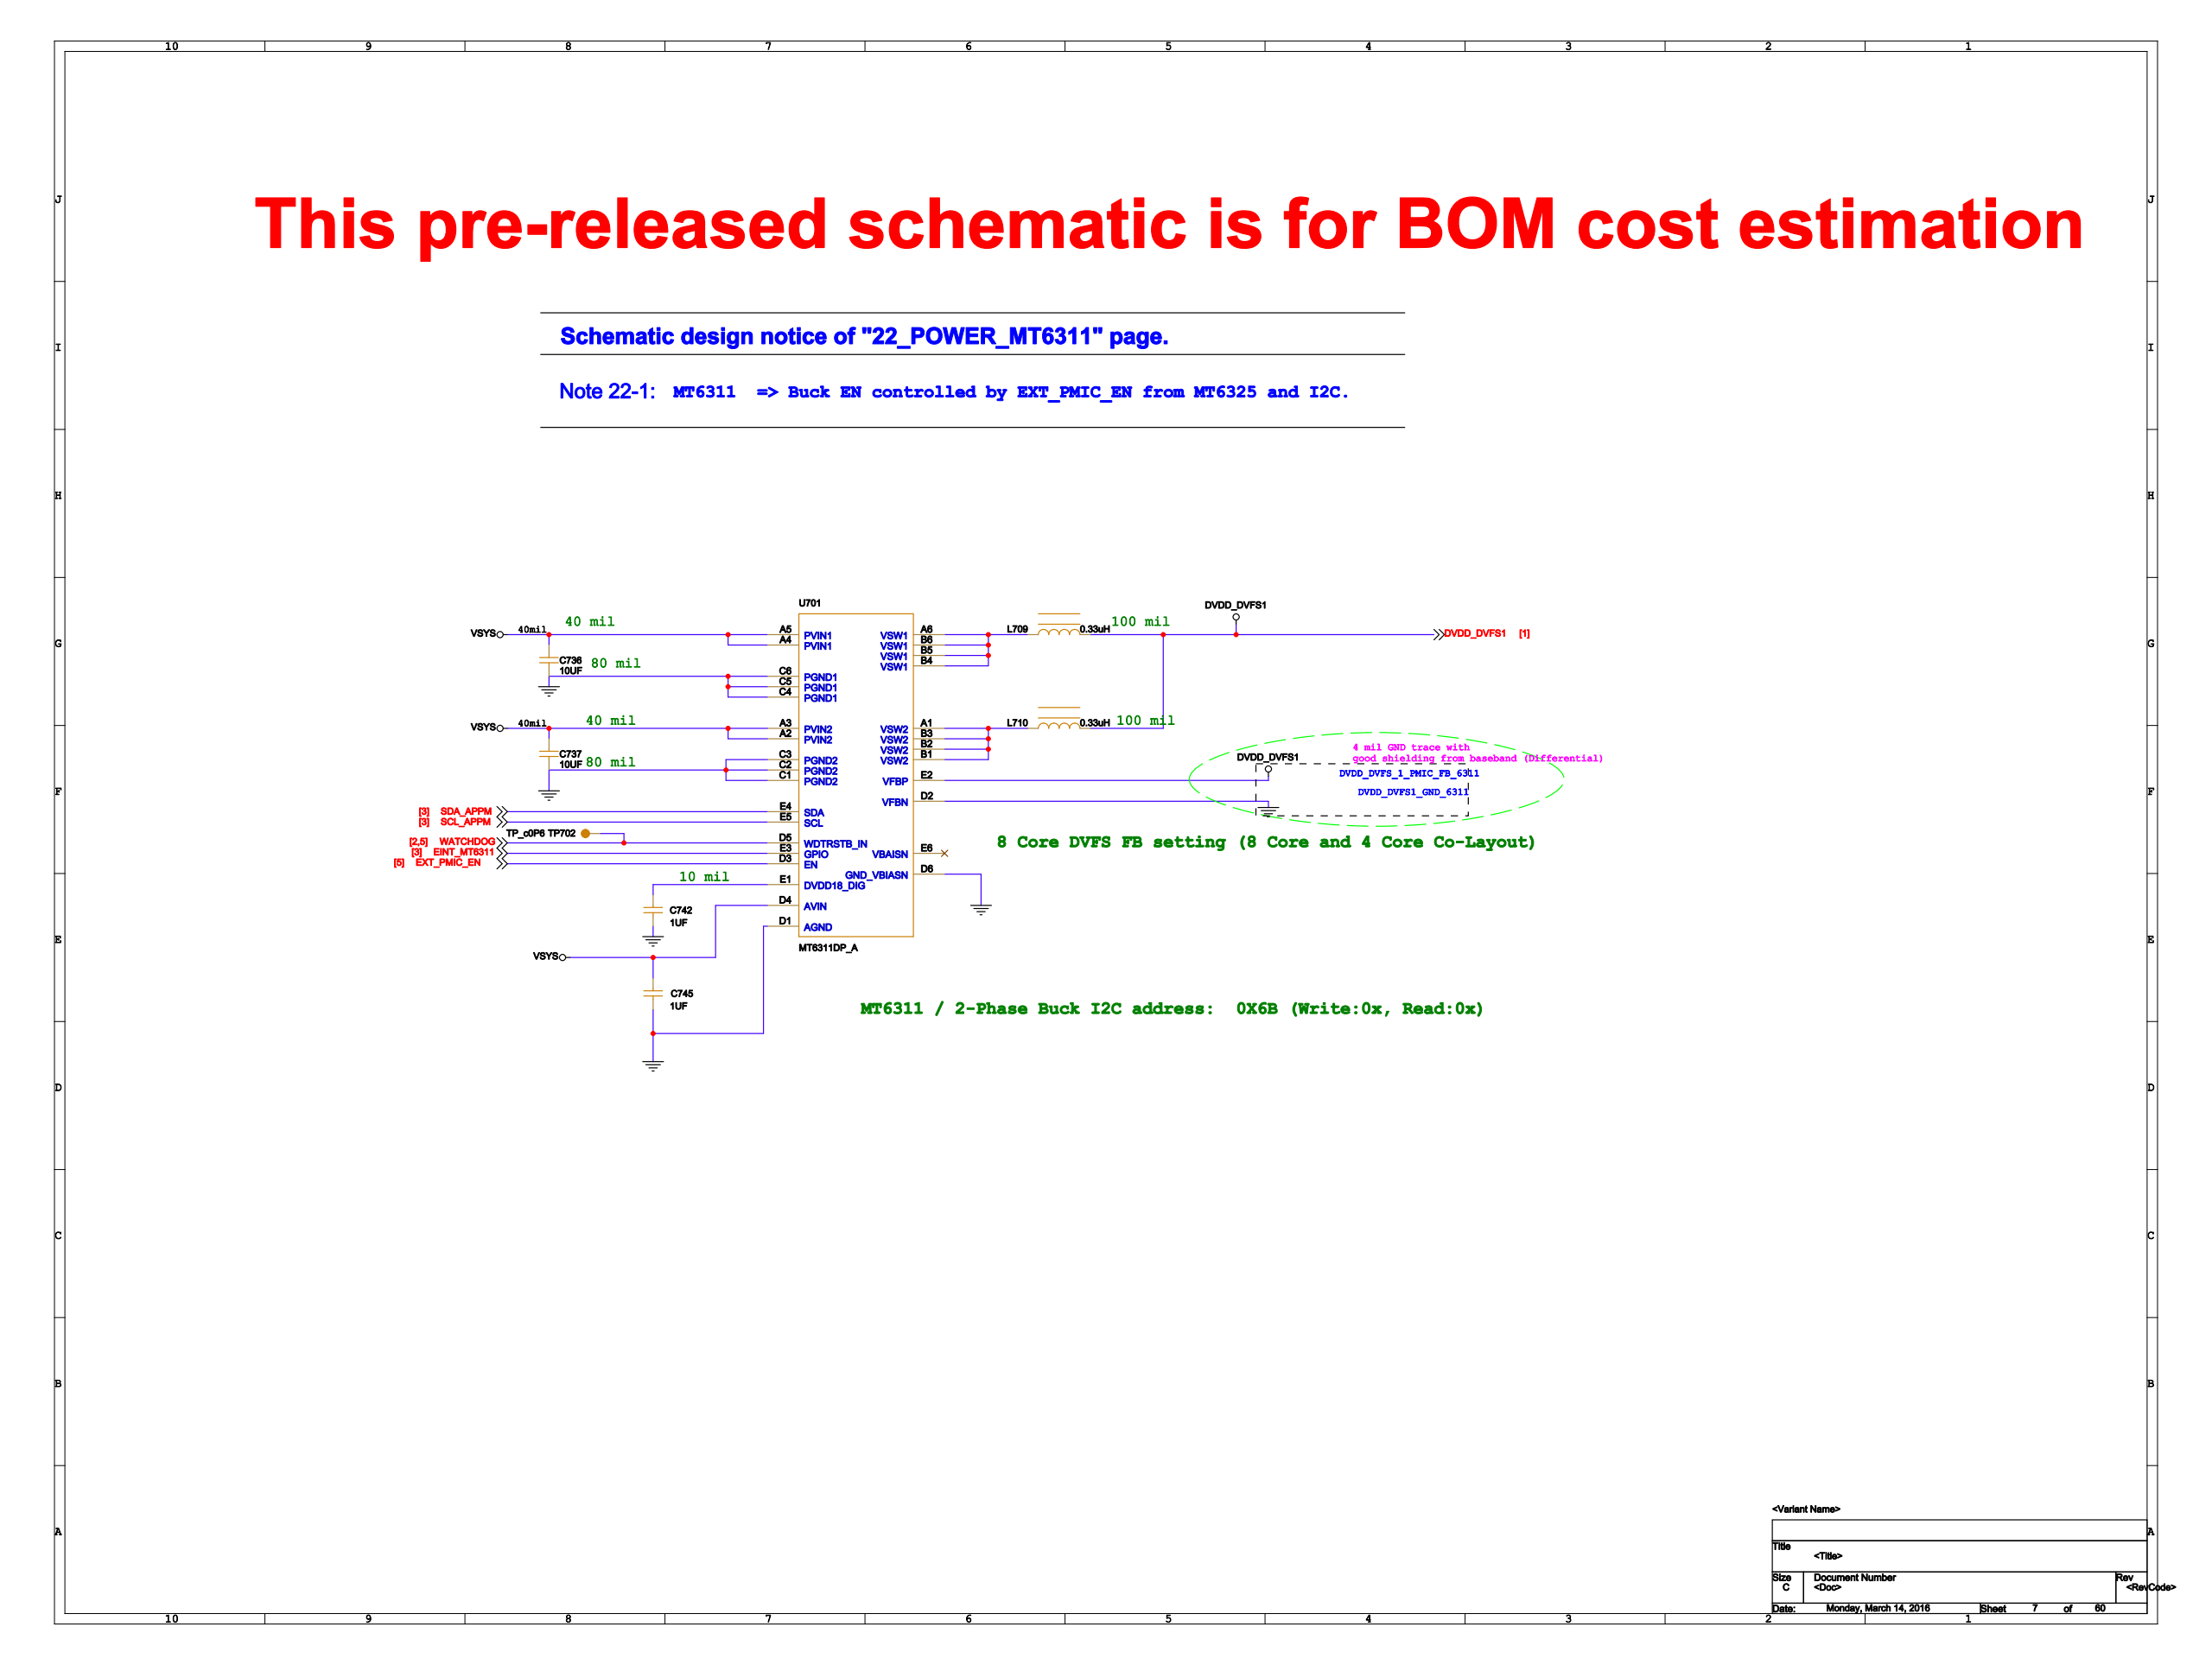Circuit board | Cadence Allegro | 1088 parts | 793 nets | one sheet of the schematic
Parts on this sheet (reference | value | footprint):
C736 | 10UF | 0402-BIG
C737 | 10UF | 0402-BIG
C742 | 1UF | C0201
C745 | 1UF | C0201
L709 | 0.33uH | L2520_MAKK2520
L710 | 0.33uH | L2520_MAKK2520
TP702 | TP_c0P6 | TP_C0P6
U701 | MT6311DP_A | MT6311
Nets of these parts (net: part-pin ...):
GND: C736-2 C737-2 C742-2 C745-2 U701-C1 U701-C2 U701-C3 U701-C4 U701-C5 U701-C6 U701-D1 U701-D2 U701-D6
VSYS: C736-1 C737-1 C745-1 U701-A2 U701-A3 U701-A4 U701-A5 U701-D4
WATCHDOG: TP702-1 U701-D5
EINT_MT6311: U701-E3
SCL_APPM: U701-E5
SDA_APPM: U701-E4
DVDD_DVFS1: L709-2 L710-2 U701-E2
N30704658: C742-1 U701-E1
EXT_PMIC_EN: U701-D3
N30704678: L709-1 U701-A6 U701-B4 U701-B5 U701-B6
N30704676: L710-1 U701-A1 U701-B1 U701-B2 U701-B3